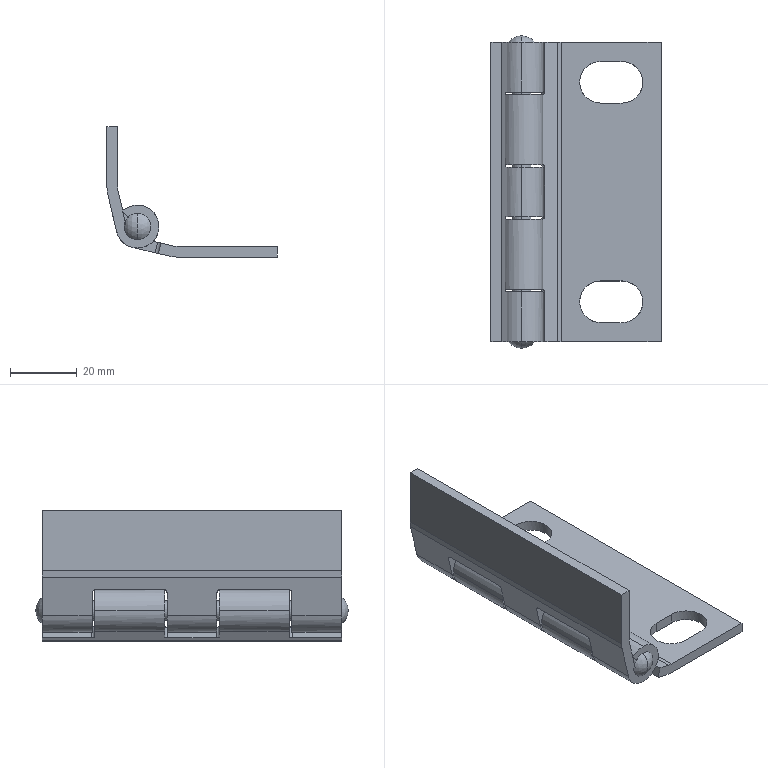Part | SolidWorks | features BaseBody 3 | 3 solids | 90 faces | box 51.2 x 94 x 39.2 mm | volume 27609 mm3 | cylinder 48 | plane 38 | sphere 4 | commonest cylinder face diameters 6.5 x15 12.9 x15 2 x8 12.5 x4 6 x2 10 x2